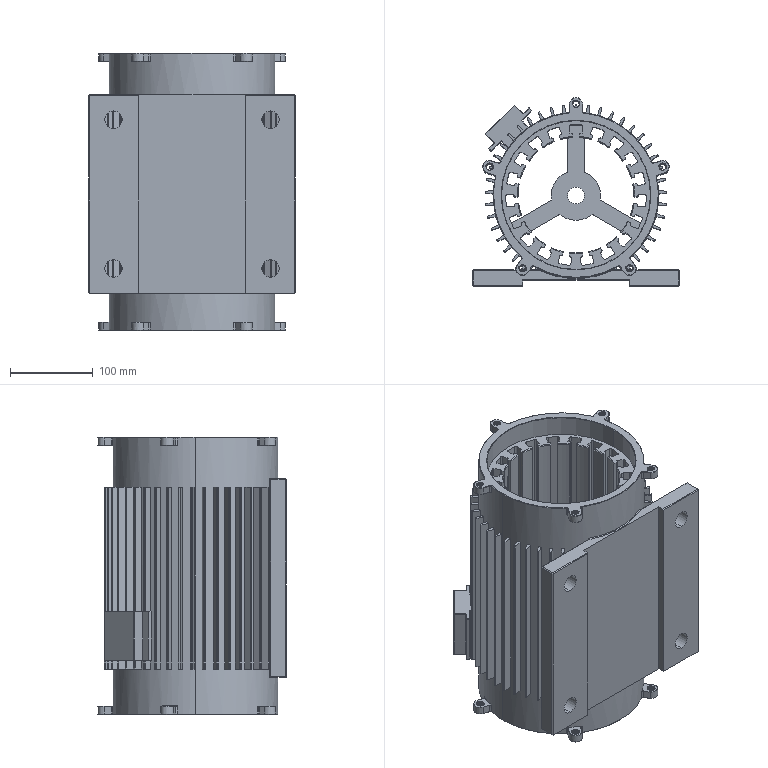Part | SolidWorks | 1 solid | 1065 faces | box 250 x 228 x 335 mm | volume 4838196 mm3 | plane 471 | cylinder 435 | cone 127 | spline 32 | commonest cylinder face diameters 8 x148 4 x100 0.769 x96 220 x39 140 x20 16 x10